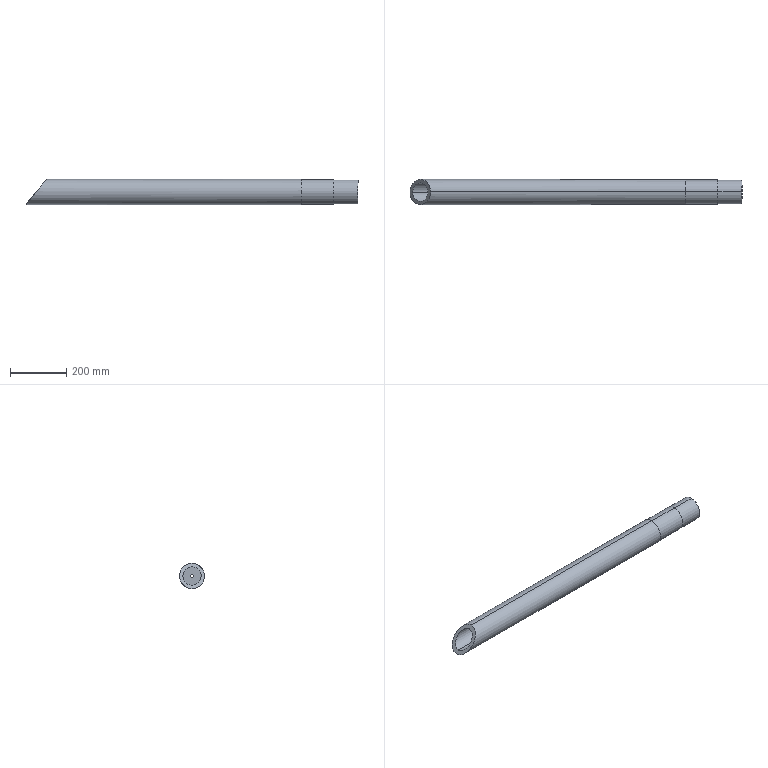Part | SolidWorks | features ICE 5, 3DProfileFeature 2, Chamfer 2, Cut 1, DelFace 1, DeleteBody 1, HoleWzd 1, RefCurve 1, Revolution 1, Split 1, SurfCut 1 | 2 solids | 22 faces | box 1176 x 89 x 89 mm | volume 3262124 mm3 | cylinder 12 | plane 6 | cone 2 | torus 2 | commonest cylinder face diameters 10.2 x2 64.8 x2 65 x2 85 x2 87 x2 89 x2
STEP:
#1=CARTESIAN_POINT('',(1038.,0.,-123.5));
#2=VERTEX_POINT('',#1);
#3=CARTESIAN_POINT('',(1038.,0.,-36.5));
#4=VERTEX_POINT('',#3);
#5=CARTESIAN_POINT('',(1038.,0.,-80.));
#6=DIRECTION('',(1.,0.,0.));
#7=DIRECTION('',(0.,0.,-1.));
#8=AXIS2_PLACEMENT_3D('',#5,#6,#7);
#9=CIRCLE('',#8,43.5);
#10=EDGE_CURVE('',#2,#4,#9,.T.);
#11=ORIENTED_EDGE('',*,*,#10,.T.);
#12=CARTESIAN_POINT('',(1151.4,0.,-36.5));
#13=VERTEX_POINT('',#12);
#14=CARTESIAN_POINT('',(1038.,0.,-36.5));
#15=DIRECTION('',(1.,0.,0.));
#16=VECTOR('',#15,1000.);
#17=LINE('',#14,#16);
#18=EDGE_CURVE('',#4,#13,#17,.T.);
#19=ORIENTED_EDGE('',*,*,#18,.T.);
#20=CARTESIAN_POINT('',(1151.4,0.,-123.5));
#21=VERTEX_POINT('',#20);
#22=CARTESIAN_POINT('',(1151.4,0.,-80.));
#23=DIRECTION('',(1.,0.,0.));
#24=DIRECTION('',(0.,0.,-1.));
#25=AXIS2_PLACEMENT_3D('',#22,#23,#24);
#26=CIRCLE('',#25,43.5);
#27=EDGE_CURVE('',#21,#13,#26,.T.);
#28=ORIENTED_EDGE('',*,*,#27,.F.);
#29=CARTESIAN_POINT('',(1038.,0.,-123.5));
#30=DIRECTION('',(1.,0.,0.));
#31=VECTOR('',#30,1000.);
#32=LINE('',#29,#31);
#33=EDGE_CURVE('',#2,#21,#32,.T.);
#34=ORIENTED_EDGE('',*,*,#33,.F.);
#35=EDGE_LOOP('',(#11,#19,#28,#34));
#36=FACE_OUTER_BOUND('',#35,.T.);
#37=CARTESIAN_POINT('',(1038.,0.,-80.));
#38=DIRECTION('',(1.,0.,0.));
#39=DIRECTION('',(0.,0.,-1.));
#40=AXIS2_PLACEMENT_3D('',#37,#38,#39);
#41=CYLINDRICAL_SURFACE('',#40,43.5);
#42=ADVANCED_FACE('',(#36),#41,.T.);
#43=CARTESIAN_POINT('',(1237.1,0.,-121.5));
#44=VERTEX_POINT('',#43);
#45=CARTESIAN_POINT('',(1237.1,0.,-38.5));
#46=VERTEX_POINT('',#45);
#47=CARTESIAN_POINT('',(1237.1,0.,-80.));
#48=DIRECTION('',(1.,0.,0.));
#49=DIRECTION('',(0.,0.,1.));
#50=AXIS2_PLACEMENT_3D('',#47,#48,#49);
#51=CIRCLE('',#50,41.5);
#52=EDGE_CURVE('',#44,#46,#51,.T.);
#53=ORIENTED_EDGE('',*,*,#52,.F.);
#54=CARTESIAN_POINT('',(1236.1,0.,-122.5));
#55=VERTEX_POINT('',#54);
#56=CARTESIAN_POINT('',(1237.1,0.,-121.5));
#57=DIRECTION('',(-0.7071,0.,-0.7071));
#58=VECTOR('',#57,1000.);
#59=LINE('',#56,#58);
#60=EDGE_CURVE('',#44,#55,#59,.T.);
#61=ORIENTED_EDGE('',*,*,#60,.T.);
#62=CARTESIAN_POINT('',(1236.1,0.,-37.5));
#63=VERTEX_POINT('',#62);
#64=CARTESIAN_POINT('',(1236.1,0.,-80.));
#65=DIRECTION('',(-1.,0.,0.));
#66=DIRECTION('',(0.,0.,1.));
#67=AXIS2_PLACEMENT_3D('',#64,#65,#66);
#68=CIRCLE('',#67,42.5);
#69=EDGE_CURVE('',#63,#55,#68,.T.);
#70=ORIENTED_EDGE('',*,*,#69,.F.);
#71=CARTESIAN_POINT('',(1237.1,0.,-38.5));
#72=DIRECTION('',(-0.7071,0.,0.7071));
#73=VECTOR('',#72,1000.);
#74=LINE('',#71,#73);
#75=EDGE_CURVE('',#46,#63,#74,.T.);
#76=ORIENTED_EDGE('',*,*,#75,.F.);
#77=EDGE_LOOP('',(#53,#61,#70,#76));
#78=FACE_OUTER_BOUND('',#77,.T.);
#79=CARTESIAN_POINT('',(1237.1,0.,-80.));
#80=DIRECTION('',(-1.,0.,0.));
#81=DIRECTION('',(0.,0.,1.));
#82=AXIS2_PLACEMENT_3D('',#79,#80,#81);
#83=CONICAL_SURFACE('',#82,41.5,0.7854);
#84=ADVANCED_FACE('',(#78),#83,.T.);
#85=CARTESIAN_POINT('',(1151.4,0.,-122.5));
#86=VERTEX_POINT('',#85);
#87=CARTESIAN_POINT('',(1151.4,0.,-37.5));
#88=VERTEX_POINT('',#87);
#89=CARTESIAN_POINT('',(1151.4,0.,-80.));
#90=DIRECTION('',(1.,0.,0.));
#91=DIRECTION('',(0.,0.,-1.));
#92=AXIS2_PLACEMENT_3D('',#89,#90,#91);
#93=CIRCLE('',#92,42.5);
#94=EDGE_CURVE('',#86,#88,#93,.T.);
#95=ORIENTED_EDGE('',*,*,#94,.T.);
#96=CARTESIAN_POINT('',(1151.4,0.,-37.5));
#97=DIRECTION('',(1.,0.,0.));
#98=VECTOR('',#97,1000.);
#99=LINE('',#96,#98);
#100=EDGE_CURVE('',#88,#63,#99,.T.);
#101=ORIENTED_EDGE('',*,*,#100,.T.);
#102=ORIENTED_EDGE('',*,*,#69,.T.);
#103=CARTESIAN_POINT('',(1151.4,0.,-122.5));
#104=DIRECTION('',(1.,0.,0.));
#105=VECTOR('',#104,1000.);
#106=LINE('',#103,#105);
#107=EDGE_CURVE('',#86,#55,#106,.T.);
#108=ORIENTED_EDGE('',*,*,#107,.F.);
#109=EDGE_LOOP('',(#95,#101,#102,#108));
#110=FACE_OUTER_BOUND('',#109,.T.);
#111=CARTESIAN_POINT('',(1151.4,0.,-80.));
#112=DIRECTION('',(1.,0.,0.));
#113=DIRECTION('',(0.,0.,-1.));
#114=AXIS2_PLACEMENT_3D('',#111,#112,#113);
#115=CYLINDRICAL_SURFACE('',#114,42.5);
#116=ADVANCED_FACE('',(#110),#115,.T.);
#117=CARTESIAN_POINT('',(1237.1,0.,-112.5));
#118=VERTEX_POINT('',#117);
#119=CARTESIAN_POINT('',(1237.1,0.,-47.5));
#120=VERTEX_POINT('',#119);
#121=CARTESIAN_POINT('',(1237.1,0.,-80.));
#122=DIRECTION('',(-1.,0.,0.));
#123=DIRECTION('',(0.,0.,1.));
#124=AXIS2_PLACEMENT_3D('',#121,#122,#123);
#125=CIRCLE('',#124,32.5);
#126=EDGE_CURVE('',#118,#120,#125,.T.);
#127=ORIENTED_EDGE('',*,*,#126,.F.);
#128=CARTESIAN_POINT('',(70.942,0.,-112.5));
#129=VERTEX_POINT('',#128);
#130=CARTESIAN_POINT('',(1237.1,0.,-112.5));
#131=DIRECTION('',(-1.,0.,0.));
#132=VECTOR('',#131,1000.);
#133=LINE('',#130,#132);
#134=EDGE_CURVE('',#118,#129,#133,.T.);
#135=ORIENTED_EDGE('',*,*,#134,.T.);
#136=CARTESIAN_POINT('',(70.94,-2.772,-112.382));
#137=VERTEX_POINT('',#136);
#138=CARTESIAN_POINT('',(70.942,0.,-112.5));
#139=CARTESIAN_POINT('',(70.942,-0.4648,-112.5));
#140=CARTESIAN_POINT('',(70.942,-0.9292,-112.49));
#141=CARTESIAN_POINT('',(70.941,-1.853,-112.45));
#142=CARTESIAN_POINT('',(70.941,-2.314,-112.421));
#143=CARTESIAN_POINT('',(70.94,-2.772,-112.382));
#144=B_SPLINE_CURVE_WITH_KNOTS('',3,(#138,#139,#140,#141,#142,#143),.UNSPECIFIED.,.F.,.F.,(4,2,4),(0.2193,0.2207,0.2221),.UNSPECIFIED.);
#145=EDGE_CURVE('',#129,#137,#144,.T.);
#146=ORIENTED_EDGE('',*,*,#145,.T.);
#147=CARTESIAN_POINT('',(124.035,-3.109,-47.649));
#148=VERTEX_POINT('',#147);
#149=CARTESIAN_POINT('',(124.035,-3.109,-47.649));
#150=CARTESIAN_POINT('',(119.734,-57.671,-52.893));
#151=CARTESIAN_POINT('',(74.775,-57.386,-107.706));
#152=CARTESIAN_POINT('',(70.94,-2.772,-112.382));
#153=(BOUNDED_CURVE()B_SPLINE_CURVE(3,(#149,#150,#151,#152),.UNSPECIFIED.,.F.,.F.)B_SPLINE_CURVE_WITH_KNOTS((4,4),(3.237,6.198),.UNSPECIFIED.)CURVE()GEOMETRIC_REPRESENTATION_ITEM()RATIONAL_B_SPLINE_CURVE((1.,0.3937,0.3937,1.))REPRESENTATION_ITEM(''));
#154=EDGE_CURVE('',#148,#137,#153,.T.);
#155=ORIENTED_EDGE('',*,*,#154,.F.);
#156=CARTESIAN_POINT('',(124.229,0.,-47.5));
#157=VERTEX_POINT('',#156);
#158=CARTESIAN_POINT('',(124.035,-3.109,-47.649));
#159=CARTESIAN_POINT('',(124.099,-2.598,-47.6));
#160=CARTESIAN_POINT('',(124.147,-2.081,-47.563));
#161=CARTESIAN_POINT('',(124.213,-1.039,-47.512));
#162=CARTESIAN_POINT('',(124.229,-0.518,-47.5));
#163=CARTESIAN_POINT('',(124.229,0.,-47.5));
#164=B_SPLINE_CURVE_WITH_KNOTS('',3,(#158,#159,#160,#161,#162,#163),.UNSPECIFIED.,.F.,.F.,(4,2,4),(0.09483,0.09637,0.09791),.UNSPECIFIED.);
#165=EDGE_CURVE('',#148,#157,#164,.T.);
#166=ORIENTED_EDGE('',*,*,#165,.T.);
#167=CARTESIAN_POINT('',(1237.1,0.,-47.5));
#168=DIRECTION('',(-1.,0.,0.));
#169=VECTOR('',#168,1000.);
#170=LINE('',#167,#169);
#171=EDGE_CURVE('',#120,#157,#170,.T.);
#172=ORIENTED_EDGE('',*,*,#171,.F.);
#173=EDGE_LOOP('',(#127,#135,#146,#155,#166,#172));
#174=FACE_OUTER_BOUND('',#173,.T.);
#175=CARTESIAN_POINT('',(1237.1,0.,-80.));
#176=DIRECTION('',(-1.,0.,0.));
#177=DIRECTION('',(0.,0.,1.));
#178=AXIS2_PLACEMENT_3D('',#175,#176,#177);
#179=CYLINDRICAL_SURFACE('',#178,32.5);
#180=ADVANCED_FACE('',(#174),#179,.F.);
#181=CARTESIAN_POINT('',(1038.,0.,-124.5));
#182=VERTEX_POINT('',#181);
#183=CARTESIAN_POINT('',(1038.,0.,-35.5));
#184=VERTEX_POINT('',#183);
#185=CARTESIAN_POINT('',(1038.,0.,-80.));
#186=DIRECTION('',(1.,0.,0.));
#187=DIRECTION('',(0.,0.,-1.));
#188=AXIS2_PLACEMENT_3D('',#185,#186,#187);
#189=CIRCLE('',#188,44.5);
#190=EDGE_CURVE('',#182,#184,#189,.T.);
#191=ORIENTED_EDGE('',*,*,#190,.F.);
#192=CARTESIAN_POINT('',(61.,0.,-124.5));
#193=VERTEX_POINT('',#192);
#194=CARTESIAN_POINT('',(1237.1,0.,-124.5));
#195=DIRECTION('',(-1.,0.,0.));
#196=VECTOR('',#195,1000.);
#197=LINE('',#194,#196);
#198=EDGE_CURVE('',#182,#193,#197,.T.);
#199=ORIENTED_EDGE('',*,*,#198,.T.);
#200=CARTESIAN_POINT('',(134.,0.,-35.5));
#201=VERTEX_POINT('',#200);
#202=CARTESIAN_POINT('',(61.,0.,-124.5));
#203=CARTESIAN_POINT('',(61.,89.,-124.5));
#204=CARTESIAN_POINT('',(134.,89.,-35.5));
#205=CARTESIAN_POINT('',(134.,0.,-35.5));
#206=(BOUNDED_CURVE()B_SPLINE_CURVE(3,(#202,#203,#204,#205),.UNSPECIFIED.,.F.,.F.)B_SPLINE_CURVE_WITH_KNOTS((4,4),(0.,3.142),.UNSPECIFIED.)CURVE()GEOMETRIC_REPRESENTATION_ITEM()RATIONAL_B_SPLINE_CURVE((1.,0.3333,0.3333,1.))REPRESENTATION_ITEM(''));
#207=EDGE_CURVE('',#193,#201,#206,.T.);
#208=ORIENTED_EDGE('',*,*,#207,.T.);
#209=CARTESIAN_POINT('',(1237.1,0.,-35.5));
#210=DIRECTION('',(-1.,0.,0.));
#211=VECTOR('',#210,1000.);
#212=LINE('',#209,#211);
#213=EDGE_CURVE('',#184,#201,#212,.T.);
#214=ORIENTED_EDGE('',*,*,#213,.F.);
#215=EDGE_LOOP('',(#191,#199,#208,#214));
#216=FACE_OUTER_BOUND('',#215,.T.);
#217=CARTESIAN_POINT('',(1237.1,0.,-80.));
#218=DIRECTION('',(-1.,0.,0.));
#219=DIRECTION('',(0.,0.,1.));
#220=AXIS2_PLACEMENT_3D('',#217,#218,#219);
#221=CYLINDRICAL_SURFACE('',#220,44.5);
#222=ADVANCED_FACE('',(#216),#221,.T.);
#223=ORIENTED_EDGE('',*,*,#198,.F.);
#224=CARTESIAN_POINT('',(1038.,0.,-80.));
#225=DIRECTION('',(1.,0.,0.));
#226=DIRECTION('',(0.,0.,-1.));
#227=AXIS2_PLACEMENT_3D('',#224,#225,#226);
#228=CIRCLE('',#227,44.5);
#229=EDGE_CURVE('',#184,#182,#228,.T.);
#230=ORIENTED_EDGE('',*,*,#229,.F.);
#231=ORIENTED_EDGE('',*,*,#213,.T.);
#232=CARTESIAN_POINT('',(134.,0.,-35.5));
#233=CARTESIAN_POINT('',(134.,-89.,-35.5));
#234=CARTESIAN_POINT('',(61.,-89.,-124.5));
#235=CARTESIAN_POINT('',(61.,0.,-124.5));
#236=(BOUNDED_CURVE()B_SPLINE_CURVE(3,(#232,#233,#234,#235),.UNSPECIFIED.,.F.,.F.)B_SPLINE_CURVE_WITH_KNOTS((4,4),(3.142,6.283),.UNSPECIFIED.)CURVE()GEOMETRIC_REPRESENTATION_ITEM()RATIONAL_B_SPLINE_CURVE((1.,0.3333,0.3333,1.))REPRESENTATION_ITEM(''));
#237=EDGE_CURVE('',#201,#193,#236,.T.);
#238=ORIENTED_EDGE('',*,*,#237,.T.);
#239=EDGE_LOOP('',(#223,#230,#231,#238));
#240=FACE_OUTER_BOUND('',#239,.T.);
#241=CARTESIAN_POINT('',(1237.1,0.,-80.));
#242=DIRECTION('',(-1.,0.,0.));
#243=DIRECTION('',(0.,0.,1.));
#244=AXIS2_PLACEMENT_3D('',#241,#242,#243);
#245=CYLINDRICAL_SURFACE('',#244,44.5);
#246=ADVANCED_FACE('',(#240),#245,.T.);
#247=ORIENTED_EDGE('',*,*,#134,.F.);
#248=CARTESIAN_POINT('',(1237.1,0.,-80.));
#249=DIRECTION('',(-1.,0.,0.));
#250=DIRECTION('',(0.,0.,1.));
#251=AXIS2_PLACEMENT_3D('',#248,#249,#250);
#252=CIRCLE('',#251,32.5);
#253=EDGE_CURVE('',#120,#118,#252,.T.);
#254=ORIENTED_EDGE('',*,*,#253,.F.);
#255=ORIENTED_EDGE('',*,*,#171,.T.);
#256=CARTESIAN_POINT('',(124.035,3.109,-47.649));
#257=VERTEX_POINT('',#256);
#258=CARTESIAN_POINT('',(124.229,0.,-47.5));
#259=CARTESIAN_POINT('',(124.229,0.5223,-47.5));
#260=CARTESIAN_POINT('',(124.196,1.563,-47.525));
#261=CARTESIAN_POINT('',(124.099,2.595,-47.6));
#262=CARTESIAN_POINT('',(124.035,3.109,-47.649));
#263=B_SPLINE_CURVE_WITH_KNOTS('',3,(#258,#259,#260,#261,#262),.UNSPECIFIED.,.F.,.F.,(4,1,4),(0.09791,0.09946,0.101),.UNSPECIFIED.);
#264=EDGE_CURVE('',#157,#257,#263,.T.);
#265=ORIENTED_EDGE('',*,*,#264,.T.);
#266=CARTESIAN_POINT('',(70.94,2.772,-112.382));
#267=VERTEX_POINT('',#266);
#268=CARTESIAN_POINT('',(70.94,2.772,-112.382));
#269=CARTESIAN_POINT('',(74.775,57.386,-107.706));
#270=CARTESIAN_POINT('',(119.734,57.671,-52.893));
#271=CARTESIAN_POINT('',(124.035,3.109,-47.649));
#272=(BOUNDED_CURVE()B_SPLINE_CURVE(3,(#268,#269,#270,#271),.UNSPECIFIED.,.F.,.T.)B_SPLINE_CURVE_WITH_KNOTS((4,4),(0.08541,3.046),.UNSPECIFIED.)CURVE()GEOMETRIC_REPRESENTATION_ITEM()RATIONAL_B_SPLINE_CURVE((1.,0.3937,0.3937,1.))REPRESENTATION_ITEM(''));
#273=EDGE_CURVE('',#267,#257,#272,.T.);
#274=ORIENTED_EDGE('',*,*,#273,.F.);
#275=CARTESIAN_POINT('',(70.94,2.772,-112.382));
#276=CARTESIAN_POINT('',(70.941,2.313,-112.421));
#277=CARTESIAN_POINT('',(70.942,1.393,-112.48));
#278=CARTESIAN_POINT('',(70.942,0.4653,-112.5));
#279=CARTESIAN_POINT('',(70.942,0.,-112.5));
#280=B_SPLINE_CURVE_WITH_KNOTS('',3,(#275,#276,#277,#278,#279),.UNSPECIFIED.,.F.,.F.,(4,1,4),(0.2166,0.2179,0.2193),.UNSPECIFIED.);
#281=EDGE_CURVE('',#267,#129,#280,.T.);
#282=ORIENTED_EDGE('',*,*,#281,.T.);
#283=EDGE_LOOP('',(#247,#254,#255,#265,#274,#282));
#284=FACE_OUTER_BOUND('',#283,.T.);
#285=CARTESIAN_POINT('',(1237.1,0.,-80.));
#286=DIRECTION('',(-1.,0.,0.));
#287=DIRECTION('',(0.,0.,1.));
#288=AXIS2_PLACEMENT_3D('',#285,#286,#287);
#289=CYLINDRICAL_SURFACE('',#288,32.5);
#290=ADVANCED_FACE('',(#284),#289,.F.);
#291=CARTESIAN_POINT('',(70.94,-2.772,-112.382));
#292=CARTESIAN_POINT('',(70.805,-1.855,-112.546));
#293=CARTESIAN_POINT('',(70.737,-0.9308,-112.629));
#294=CARTESIAN_POINT('',(70.737,0.4579,-112.629));
#295=CARTESIAN_POINT('',(70.754,0.9216,-112.609));
#296=CARTESIAN_POINT('',(70.821,1.851,-112.526));
#297=CARTESIAN_POINT('',(70.873,2.317,-112.463));
#298=CARTESIAN_POINT('',(70.94,2.772,-112.382));
#299=B_SPLINE_CURVE_WITH_KNOTS('',3,(#291,#292,#293,#294,#295,#296,#297,#298),.UNSPECIFIED.,.F.,.F.,(4,2,2,4),(0.0102,0.01299,0.01438,0.01577),.UNSPECIFIED.);
#300=EDGE_CURVE('',#137,#267,#299,.T.);
#301=ORIENTED_EDGE('',*,*,#300,.F.);
#302=ORIENTED_EDGE('',*,*,#145,.F.);
#303=ORIENTED_EDGE('',*,*,#281,.F.);
#304=EDGE_LOOP('',(#301,#302,#303));
#305=FACE_OUTER_BOUND('',#304,.T.);
#306=CARTESIAN_POINT('',(0.,0.,0.));
#307=DIRECTION('',(0.,-1.,0.));
#308=DIRECTION('',(0.,0.,-1.));
#309=AXIS2_PLACEMENT_3D('',#306,#307,#308);
#310=TOROIDAL_SURFACE('',#309,95.,38.);
#311=ADVANCED_FACE('',(#305),#310,.F.);
#312=CARTESIAN_POINT('',(124.035,3.109,-47.649));
#313=CARTESIAN_POINT('',(124.118,2.605,-47.547));
#314=CARTESIAN_POINT('',(124.183,2.088,-47.469));
#315=CARTESIAN_POINT('',(124.27,1.039,-47.363));
#316=CARTESIAN_POINT('',(124.291,0.5167,-47.337));
#317=CARTESIAN_POINT('',(124.291,-0.5253,-47.338));
#318=CARTESIAN_POINT('',(124.269,-1.045,-47.364));
#319=CARTESIAN_POINT('',(124.184,-2.08,-47.468));
#320=CARTESIAN_POINT('',(124.12,-2.598,-47.546));
#321=CARTESIAN_POINT('',(124.035,-3.109,-47.649));
#322=B_SPLINE_CURVE_WITH_KNOTS('',3,(#312,#313,#314,#315,#316,#317,#318,#319,#320,#321),.UNSPECIFIED.,.F.,.F.,(4,2,2,2,4),(0.1138,0.1153,0.1169,0.1185,0.12),.UNSPECIFIED.);
#323=EDGE_CURVE('',#257,#148,#322,.T.);
#324=ORIENTED_EDGE('',*,*,#323,.F.);
#325=ORIENTED_EDGE('',*,*,#264,.F.);
#326=ORIENTED_EDGE('',*,*,#165,.F.);
#327=EDGE_LOOP('',(#324,#325,#326));
#328=FACE_OUTER_BOUND('',#327,.T.);
#329=CARTESIAN_POINT('',(0.,0.,0.));
#330=DIRECTION('',(0.,-1.,0.));
#331=DIRECTION('',(0.,0.,-1.));
#332=AXIS2_PLACEMENT_3D('',#329,#330,#331);
#333=TOROIDAL_SURFACE('',#332,95.,38.);
#334=ADVANCED_FACE('',(#328),#333,.F.);
#335=ORIENTED_EDGE('',*,*,#94,.F.);
#336=CARTESIAN_POINT('',(1151.4,0.,-80.));
#337=DIRECTION('',(1.,0.,0.));
#338=DIRECTION('',(0.,0.,-1.));
#339=AXIS2_PLACEMENT_3D('',#336,#337,#338);
#340=CIRCLE('',#339,42.5);
#341=EDGE_CURVE('',#88,#86,#340,.T.);
#342=ORIENTED_EDGE('',*,*,#341,.F.);
#343=EDGE_LOOP('',(#335,#342));
#344=FACE_BOUND('',#343,.T.);
#345=ORIENTED_EDGE('',*,*,#27,.T.);
#346=CARTESIAN_POINT('',(1151.4,0.,-80.));
#347=DIRECTION('',(1.,0.,0.));
#348=DIRECTION('',(0.,0.,-1.));
#349=AXIS2_PLACEMENT_3D('',#346,#347,#348);
#350=CIRCLE('',#349,43.5);
#351=EDGE_CURVE('',#13,#21,#350,.T.);
#352=ORIENTED_EDGE('',*,*,#351,.T.);
#353=EDGE_LOOP('',(#345,#352));
#354=FACE_OUTER_BOUND('',#353,.T.);
#355=CARTESIAN_POINT('',(1151.4,0.,-80.));
#356=DIRECTION('',(1.,0.,0.));
#357=DIRECTION('',(0.,0.,-1.));
#358=AXIS2_PLACEMENT_3D('',#355,#356,#357);
#359=PLANE('',#358);
#360=ADVANCED_FACE('',(#344,#354),#359,.T.);
#361=CARTESIAN_POINT('',(1237.1,0.,-80.));
#362=DIRECTION('',(1.,0.,0.));
#363=DIRECTION('',(0.,0.,1.));
#364=AXIS2_PLACEMENT_3D('',#361,#362,#363);
#365=CIRCLE('',#364,41.5);
#366=EDGE_CURVE('',#46,#44,#365,.T.);
#367=ORIENTED_EDGE('',*,*,#366,.T.);
#368=ORIENTED_EDGE('',*,*,#52,.T.);
#369=EDGE_LOOP('',(#367,#368));
#370=FACE_OUTER_BOUND('',#369,.T.);
#371=ORIENTED_EDGE('',*,*,#253,.T.);
#372=ORIENTED_EDGE('',*,*,#126,.T.);
#373=EDGE_LOOP('',(#371,#372));
#374=FACE_BOUND('',#373,.T.);
#375=CARTESIAN_POINT('',(1237.1,0.,-80.));
#376=DIRECTION('',(-1.,0.,0.));
#377=DIRECTION('',(0.,0.,1.));
#378=AXIS2_PLACEMENT_3D('',#375,#376,#377);
#379=PLANE('',#378);
#380=ADVANCED_FACE('',(#370,#374),#379,.F.);
#381=ORIENTED_EDGE('',*,*,#100,.F.);
#382=ORIENTED_EDGE('',*,*,#341,.T.);
#383=ORIENTED_EDGE('',*,*,#107,.T.);
#384=CARTESIAN_POINT('',(1236.1,0.,-80.));
#385=DIRECTION('',(-1.,0.,0.));
#386=DIRECTION('',(0.,0.,1.));
#387=AXIS2_PLACEMENT_3D('',#384,#385,#386);
#388=CIRCLE('',#387,42.5);
#389=EDGE_CURVE('',#55,#63,#388,.T.);
#390=ORIENTED_EDGE('',*,*,#389,.T.);
#391=EDGE_LOOP('',(#381,#382,#383,#390));
#392=FACE_OUTER_BOUND('',#391,.T.);
#393=CARTESIAN_POINT('',(1151.4,0.,-80.));
#394=DIRECTION('',(1.,0.,0.));
#395=DIRECTION('',(0.,0.,-1.));
#396=AXIS2_PLACEMENT_3D('',#393,#394,#395);
#397=CYLINDRICAL_SURFACE('',#396,42.5);
#398=ADVANCED_FACE('',(#392),#397,.T.);
#399=ORIENTED_EDGE('',*,*,#60,.F.);
#400=ORIENTED_EDGE('',*,*,#366,.F.);
#401=ORIENTED_EDGE('',*,*,#75,.T.);
#402=ORIENTED_EDGE('',*,*,#389,.F.);
#403=EDGE_LOOP('',(#399,#400,#401,#402));
#404=FACE_OUTER_BOUND('',#403,.T.);
#405=CARTESIAN_POINT('',(1237.1,0.,-80.));
#406=DIRECTION('',(-1.,0.,0.));
#407=DIRECTION('',(0.,0.,1.));
#408=AXIS2_PLACEMENT_3D('',#405,#406,#407);
#409=CONICAL_SURFACE('',#408,41.5,0.7854);
#410=ADVANCED_FACE('',(#404),#409,.T.);
#411=ORIENTED_EDGE('',*,*,#10,.F.);
#412=CARTESIAN_POINT('',(1038.,0.,-80.));
#413=DIRECTION('',(1.,0.,0.));
#414=DIRECTION('',(0.,0.,-1.));
#415=AXIS2_PLACEMENT_3D('',#412,#413,#414);
#416=CIRCLE('',#415,43.5);
#417=EDGE_CURVE('',#4,#2,#416,.T.);
#418=ORIENTED_EDGE('',*,*,#417,.F.);
#419=EDGE_LOOP('',(#411,#418));
#420=FACE_BOUND('',#419,.T.);
#421=ORIENTED_EDGE('',*,*,#229,.T.);
#422=ORIENTED_EDGE('',*,*,#190,.T.);
#423=EDGE_LOOP('',(#421,#422));
#424=FACE_OUTER_BOUND('',#423,.T.);
#425=CARTESIAN_POINT('',(1038.,0.,-80.));
#426=DIRECTION('',(1.,0.,0.));
#427=DIRECTION('',(0.,0.,-1.));
#428=AXIS2_PLACEMENT_3D('',#425,#426,#427);
#429=PLANE('',#428);
#430=ADVANCED_FACE('',(#420,#424),#429,.T.);
#431=ORIENTED_EDGE('',*,*,#18,.F.);
#432=ORIENTED_EDGE('',*,*,#417,.T.);
#433=ORIENTED_EDGE('',*,*,#33,.T.);
#434=ORIENTED_EDGE('',*,*,#351,.F.);
#435=EDGE_LOOP('',(#431,#432,#433,#434));
#436=FACE_OUTER_BOUND('',#435,.T.);
#437=CARTESIAN_POINT('',(1038.,0.,-80.));
#438=DIRECTION('',(1.,0.,0.));
#439=DIRECTION('',(0.,0.,-1.));
#440=AXIS2_PLACEMENT_3D('',#437,#438,#439);
#441=CYLINDRICAL_SURFACE('',#440,43.5);
#442=ADVANCED_FACE('',(#436),#441,.T.);
#443=ORIENTED_EDGE('',*,*,#237,.F.);
#444=ORIENTED_EDGE('',*,*,#207,.F.);
#445=EDGE_LOOP('',(#443,#444));
#446=FACE_OUTER_BOUND('',#445,.T.);
#447=ORIENTED_EDGE('',*,*,#154,.T.);
#448=ORIENTED_EDGE('',*,*,#300,.T.);
#449=ORIENTED_EDGE('',*,*,#273,.T.);
#450=ORIENTED_EDGE('',*,*,#323,.T.);
#451=EDGE_LOOP('',(#447,#448,#449,#450));
#452=FACE_BOUND('',#451,.T.);
#453=CARTESIAN_POINT('',(134.,1529.424,-35.5));
#454=DIRECTION('',(-0.7732,0.,0.6342));
#455=DIRECTION('',(0.6342,0.,0.7732));
#456=AXIS2_PLACEMENT_3D('',#453,#454,#455);
#457=PLANE('',#456);
#458=ADVANCED_FACE('',(#446,#452),#457,.T.);
#459=CLOSED_SHELL('',(#42,#84,#116,#180,#222,#246,#290,#311,#334,#360,#380,#398,#410,#430,#442,#458));
#460=MANIFOLD_SOLID_BREP('',#459);
#461=CARTESIAN_POINT('',(1222.1,0.,-74.9));
#462=VERTEX_POINT('',#461);
#463=CARTESIAN_POINT('',(1222.1,0.,-85.1));
#464=VERTEX_POINT('',#463);
#465=CARTESIAN_POINT('',(1222.1,0.,-80.));
#466=DIRECTION('',(1.,0.,0.));
#467=DIRECTION('',(0.,0.,-1.));
#468=AXIS2_PLACEMENT_3D('',#465,#466,#467);
#469=CIRCLE('',#468,5.1);
#470=EDGE_CURVE('',#462,#464,#469,.T.);
#471=ORIENTED_EDGE('',*,*,#470,.F.);
#472=CARTESIAN_POINT('',(1232.1,0.,-74.9));
#473=VERTEX_POINT('',#472);
#474=CARTESIAN_POINT('',(1232.1,0.,-74.9));
#475=DIRECTION('',(1.,0.,0.));
#476=VECTOR('',#475,1000.);
#477=LINE('',#474,#476);
#478=EDGE_CURVE('',#462,#473,#477,.T.);
#479=ORIENTED_EDGE('',*,*,#478,.T.);
#480=CARTESIAN_POINT('',(1232.1,0.,-85.1));
#481=VERTEX_POINT('',#480);
#482=CARTESIAN_POINT('',(1232.1,0.,-80.));
#483=DIRECTION('',(1.,0.,0.));
#484=DIRECTION('',(0.,0.,-1.));
#485=AXIS2_PLACEMENT_3D('',#482,#483,#484);
#486=CIRCLE('',#485,5.1);
#487=EDGE_CURVE('',#473,#481,#486,.T.);
#488=ORIENTED_EDGE('',*,*,#487,.T.);
#489=CARTESIAN_POINT('',(1232.1,0.,-85.1));
#490=DIRECTION('',(1.,0.,0.));
#491=VECTOR('',#490,1000.);
#492=LINE('',#489,#491);
#493=EDGE_CURVE('',#464,#481,#492,.T.);
#494=ORIENTED_EDGE('',*,*,#493,.F.);
#495=EDGE_LOOP('',(#471,#479,#488,#494));
#496=FACE_OUTER_BOUND('',#495,.T.);
#497=CARTESIAN_POINT('',(1232.1,0.,-80.));
#498=DIRECTION('',(1.,0.,0.));
#499=DIRECTION('',(0.,0.,-1.));
#500=AXIS2_PLACEMENT_3D('',#497,#498,#499);
#501=CYLINDRICAL_SURFACE('',#500,5.1);
#502=ADVANCED_FACE('',(#496),#501,.F.);
#503=CARTESIAN_POINT('',(1222.1,0.,-112.4));
#504=VERTEX_POINT('',#503);
#505=CARTESIAN_POINT('',(1222.1,0.,-47.6));
#506=VERTEX_POINT('',#505);
#507=CARTESIAN_POINT('',(1222.1,0.,-80.));
#508=DIRECTION('',(1.,0.,0.));
#509=DIRECTION('',(0.,0.,-1.));
#510=AXIS2_PLACEMENT_3D('',#507,#508,#509);
#511=CIRCLE('',#510,32.4);
#512=EDGE_CURVE('',#504,#506,#511,.T.);
#513=ORIENTED_EDGE('',*,*,#512,.T.);
#514=CARTESIAN_POINT('',(1232.1,0.,-47.6));
#515=VERTEX_POINT('',#514);
#516=CARTESIAN_POINT('',(1222.1,0.,-47.6));
#517=DIRECTION('',(1.,0.,0.));
#518=VECTOR('',#517,1000.);
#519=LINE('',#516,#518);
#520=EDGE_CURVE('',#506,#515,#519,.T.);
#521=ORIENTED_EDGE('',*,*,#520,.T.);
#522=CARTESIAN_POINT('',(1232.1,0.,-112.4));
#523=VERTEX_POINT('',#522);
#524=CARTESIAN_POINT('',(1232.1,0.,-80.));
#525=DIRECTION('',(1.,0.,0.));
#526=DIRECTION('',(0.,0.,-1.));
#527=AXIS2_PLACEMENT_3D('',#524,#525,#526);
#528=CIRCLE('',#527,32.4);
#529=EDGE_CURVE('',#523,#515,#528,.T.);
#530=ORIENTED_EDGE('',*,*,#529,.F.);
#531=CARTESIAN_POINT('',(1222.1,0.,-112.4));
#532=DIRECTION('',(1.,0.,0.));
#533=VECTOR('',#532,1000.);
#534=LINE('',#531,#533);
#535=EDGE_CURVE('',#504,#523,#534,.T.);
#536=ORIENTED_EDGE('',*,*,#535,.F.);
#537=EDGE_LOOP('',(#513,#521,#530,#536));
#538=FACE_OUTER_BOUND('',#537,.T.);
#539=CARTESIAN_POINT('',(1222.1,0.,-80.));
#540=DIRECTION('',(1.,0.,0.));
#541=DIRECTION('',(0.,0.,-1.));
#542=AXIS2_PLACEMENT_3D('',#539,#540,#541);
#543=CYLINDRICAL_SURFACE('',#542,32.4);
#544=ADVANCED_FACE('',(#538),#543,.T.);
#545=ORIENTED_EDGE('',*,*,#520,.F.);
#546=CARTESIAN_POINT('',(1222.1,0.,-80.));
#547=DIRECTION('',(1.,0.,0.));
#548=DIRECTION('',(0.,0.,-1.));
#549=AXIS2_PLACEMENT_3D('',#546,#547,#548);
#550=CIRCLE('',#549,32.4);
#551=EDGE_CURVE('',#506,#504,#550,.T.);
#552=ORIENTED_EDGE('',*,*,#551,.T.);
#553=ORIENTED_EDGE('',*,*,#535,.T.);
#554=CARTESIAN_POINT('',(1232.1,0.,-80.));
#555=DIRECTION('',(1.,0.,0.));
#556=DIRECTION('',(0.,0.,-1.));
#557=AXIS2_PLACEMENT_3D('',#554,#555,#556);
#558=CIRCLE('',#557,32.4);
#559=EDGE_CURVE('',#515,#523,#558,.T.);
#560=ORIENTED_EDGE('',*,*,#559,.F.);
#561=EDGE_LOOP('',(#545,#552,#553,#560));
#562=FACE_OUTER_BOUND('',#561,.T.);
#563=CARTESIAN_POINT('',(1222.1,0.,-80.));
#564=DIRECTION('',(1.,0.,0.));
#565=DIRECTION('',(0.,0.,-1.));
#566=AXIS2_PLACEMENT_3D('',#563,#564,#565);
#567=CYLINDRICAL_SURFACE('',#566,32.4);
#568=ADVANCED_FACE('',(#562),#567,.T.);
#569=CARTESIAN_POINT('',(1222.1,0.,-80.));
#570=DIRECTION('',(1.,0.,0.));
#571=DIRECTION('',(0.,0.,-1.));
#572=AXIS2_PLACEMENT_3D('',#569,#570,#571);
#573=CIRCLE('',#572,5.1);
#574=EDGE_CURVE('',#464,#462,#573,.T.);
#575=ORIENTED_EDGE('',*,*,#574,.T.);
#576=ORIENTED_EDGE('',*,*,#470,.T.);
#577=EDGE_LOOP('',(#575,#576));
#578=FACE_BOUND('',#577,.T.);
#579=ORIENTED_EDGE('',*,*,#512,.F.);
#580=ORIENTED_EDGE('',*,*,#551,.F.);
#581=EDGE_LOOP('',(#579,#580));
#582=FACE_OUTER_BOUND('',#581,.T.);
#583=CARTESIAN_POINT('',(1222.1,0.,-80.));
#584=DIRECTION('',(1.,0.,0.));
#585=DIRECTION('',(0.,0.,-1.));
#586=AXIS2_PLACEMENT_3D('',#583,#584,#585);
#587=PLANE('',#586);
#588=ADVANCED_FACE('',(#578,#582),#587,.F.);
#589=CARTESIAN_POINT('',(1232.1,0.,-80.));
#590=DIRECTION('',(1.,0.,0.));
#591=DIRECTION('',(0.,0.,-1.));
#592=AXIS2_PLACEMENT_3D('',#589,#590,#591);
#593=CIRCLE('',#592,5.1);
#594=EDGE_CURVE('',#481,#473,#593,.T.);
#595=ORIENTED_EDGE('',*,*,#594,.F.);
#596=ORIENTED_EDGE('',*,*,#487,.F.);
#597=EDGE_LOOP('',(#595,#596));
#598=FACE_BOUND('',#597,.T.);
#599=ORIENTED_EDGE('',*,*,#529,.T.);
#600=ORIENTED_EDGE('',*,*,#559,.T.);
#601=EDGE_LOOP('',(#599,#600));
#602=FACE_OUTER_BOUND('',#601,.T.);
#603=CARTESIAN_POINT('',(1232.1,0.,-80.));
#604=DIRECTION('',(1.,0.,0.));
#605=DIRECTION('',(0.,0.,-1.));
#606=AXIS2_PLACEMENT_3D('',#603,#604,#605);
#607=PLANE('',#606);
#608=ADVANCED_FACE('',(#598,#602),#607,.T.);
#609=ORIENTED_EDGE('',*,*,#478,.F.);
#610=ORIENTED_EDGE('',*,*,#574,.F.);
#611=ORIENTED_EDGE('',*,*,#493,.T.);
#612=ORIENTED_EDGE('',*,*,#594,.T.);
#613=EDGE_LOOP('',(#609,#610,#611,#612));
#614=FACE_OUTER_BOUND('',#613,.T.);
#615=CARTESIAN_POINT('',(1232.1,0.,-80.));
#616=DIRECTION('',(1.,0.,0.));
#617=DIRECTION('',(0.,0.,-1.));
#618=AXIS2_PLACEMENT_3D('',#615,#616,#617);
#619=CYLINDRICAL_SURFACE('',#618,5.1);
#620=ADVANCED_FACE('',(#614),#619,.F.);
#621=CLOSED_SHELL('',(#502,#544,#568,#588,#608,#620));
#622=MANIFOLD_SOLID_BREP('',#621);
#623=CARTESIAN_POINT('',(0.,0.,0.));
#624=DIRECTION('',(0.,0.,1.));
#625=DIRECTION('',(1.,0.,0.));
#626=AXIS2_PLACEMENT_3D('',#623,#624,#625);
#627=(LENGTH_UNIT()NAMED_UNIT(*)SI_UNIT(.MILLI.,.METRE.));
#628=UNCERTAINTY_MEASURE_WITH_UNIT(LENGTH_MEASURE(0.00001),#627,'','');
#629=(NAMED_UNIT(*)PLANE_ANGLE_UNIT()SI_UNIT($,.RADIAN.));
#630=(NAMED_UNIT(*)SI_UNIT($,.STERADIAN.)SOLID_ANGLE_UNIT());
#631=(GEOMETRIC_REPRESENTATION_CONTEXT(3)GLOBAL_UNCERTAINTY_ASSIGNED_CONTEXT((#628))GLOBAL_UNIT_ASSIGNED_CONTEXT((#627,#629,#630))REPRESENTATION_CONTEXT('',''));
#632=ADVANCED_BREP_SHAPE_REPRESENTATION('',(#460,#622,#626),#631);